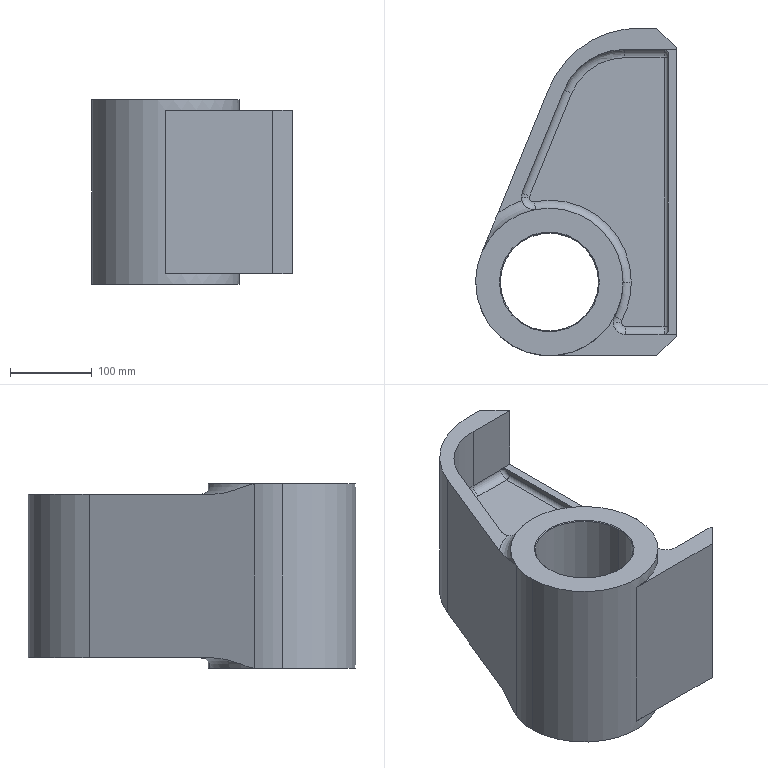Part | SolidWorks | features Fillet 4, ICE 4, Chamfer 2, Extrusion 1 | 1 solid | 77 faces | box 245 x 400 x 225 mm | volume 5993889 mm3 | cylinder 29 | plane 24 | torus 20 | cone 4 | commonest cylinder face diameters 30 x8 10 x6 20 x6 180 x4 120 x2 160 x2